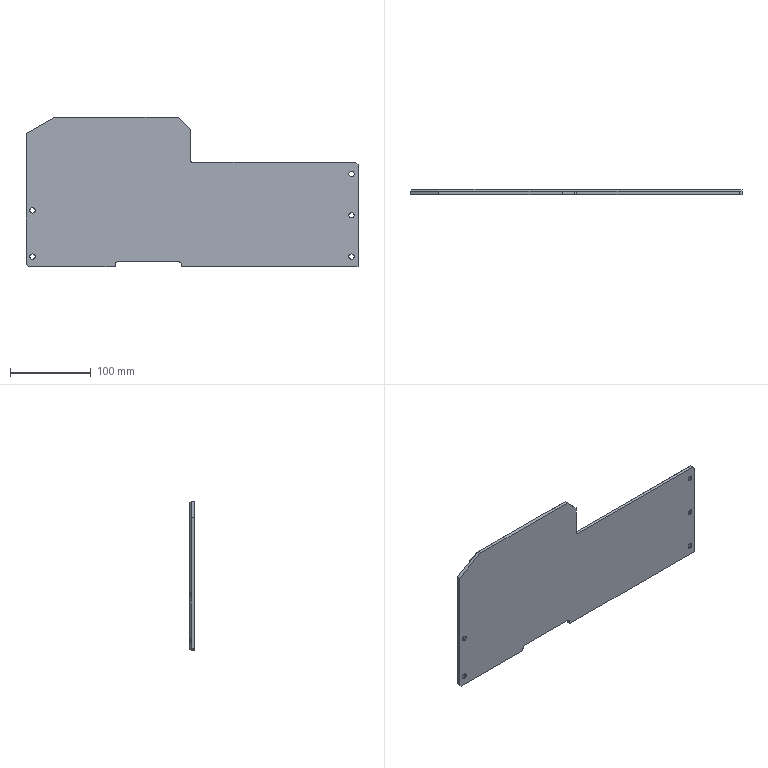Part | Creo | 1 solid | 67 faces | box 410 x 6 x 184.5 mm | volume 374225 mm3 | plane 31 | cylinder 23 | cone 13 | commonest cylinder face diameters 6.6 x10 13 x10 10 x2 6 x1